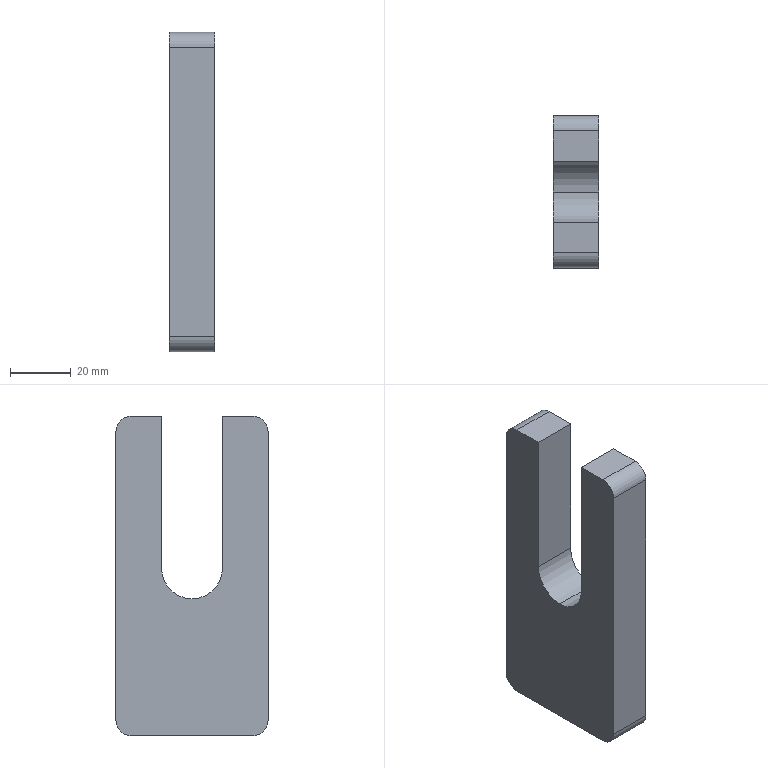Part | SolidWorks | features BaseBody 1 | 1 solid | 15 faces | box 15 x 50 x 105 mm | volume 61072 mm3 | plane 9 | cylinder 6 | commonest cylinder face diameters 10 x4 20 x2
STEP:
#1=CARTESIAN_POINT('',(0.,25.,-60.));
#2=VERTEX_POINT('',#1);
#3=CARTESIAN_POINT('',(0.,35.,-50.));
#4=VERTEX_POINT('',#3);
#5=CARTESIAN_POINT('',(0.,25.,-50.));
#6=DIRECTION('',(1.,0.,0.));
#7=DIRECTION('',(0.,0.,-1.));
#8=AXIS2_PLACEMENT_3D('',#5,#6,#7);
#9=CIRCLE('',#8,10.);
#10=EDGE_CURVE('',#2,#4,#9,.T.);
#11=ORIENTED_EDGE('',*,*,#10,.F.);
#12=CARTESIAN_POINT('',(15.,25.,-60.));
#13=VERTEX_POINT('',#12);
#14=CARTESIAN_POINT('',(0.,25.,-60.));
#15=DIRECTION('',(1.,0.,0.));
#16=VECTOR('',#15,1000.);
#17=LINE('',#14,#16);
#18=EDGE_CURVE('',#2,#13,#17,.T.);
#19=ORIENTED_EDGE('',*,*,#18,.T.);
#20=CARTESIAN_POINT('',(15.,35.,-50.));
#21=VERTEX_POINT('',#20);
#22=CARTESIAN_POINT('',(15.,25.,-50.));
#23=DIRECTION('',(-1.,0.,0.));
#24=DIRECTION('',(0.,0.,-1.));
#25=AXIS2_PLACEMENT_3D('',#22,#23,#24);
#26=CIRCLE('',#25,10.);
#27=EDGE_CURVE('',#21,#13,#26,.T.);
#28=ORIENTED_EDGE('',*,*,#27,.F.);
#29=CARTESIAN_POINT('',(0.,35.,-50.));
#30=DIRECTION('',(1.,0.,0.));
#31=VECTOR('',#30,1000.);
#32=LINE('',#29,#31);
#33=EDGE_CURVE('',#4,#21,#32,.T.);
#34=ORIENTED_EDGE('',*,*,#33,.F.);
#35=EDGE_LOOP('',(#11,#19,#28,#34));
#36=FACE_OUTER_BOUND('',#35,.T.);
#37=CARTESIAN_POINT('',(0.,25.,-50.));
#38=DIRECTION('',(1.,0.,0.));
#39=DIRECTION('',(0.,0.,-1.));
#40=AXIS2_PLACEMENT_3D('',#37,#38,#39);
#41=CYLINDRICAL_SURFACE('',#40,10.);
#42=ADVANCED_FACE('',(#36),#41,.F.);
#43=CARTESIAN_POINT('',(0.,15.,-50.));
#44=VERTEX_POINT('',#43);
#45=CARTESIAN_POINT('',(0.,25.,-50.));
#46=DIRECTION('',(1.,0.,0.));
#47=DIRECTION('',(0.,0.,-1.));
#48=AXIS2_PLACEMENT_3D('',#45,#46,#47);
#49=CIRCLE('',#48,10.);
#50=EDGE_CURVE('',#44,#2,#49,.T.);
#51=ORIENTED_EDGE('',*,*,#50,.T.);
#52=ORIENTED_EDGE('',*,*,#10,.T.);
#53=CARTESIAN_POINT('',(0.,35.,0.));
#54=VERTEX_POINT('',#53);
#55=CARTESIAN_POINT('',(0.,35.,0.));
#56=DIRECTION('',(0.,0.,1.));
#57=VECTOR('',#56,1000.);
#58=LINE('',#55,#57);
#59=EDGE_CURVE('',#4,#54,#58,.T.);
#60=ORIENTED_EDGE('',*,*,#59,.T.);
#61=CARTESIAN_POINT('',(0.,45.,0.));
#62=VERTEX_POINT('',#61);
#63=CARTESIAN_POINT('',(0.,0.,0.));
#64=DIRECTION('',(0.,1.,0.));
#65=VECTOR('',#64,1000.);
#66=LINE('',#63,#65);
#67=EDGE_CURVE('',#54,#62,#66,.T.);
#68=ORIENTED_EDGE('',*,*,#67,.T.);
#69=CARTESIAN_POINT('',(0.,50.,-5.));
#70=VERTEX_POINT('',#69);
#71=CARTESIAN_POINT('',(0.,45.,-5.));
#72=DIRECTION('',(-1.,0.,0.));
#73=DIRECTION('',(0.,0.,1.));
#74=AXIS2_PLACEMENT_3D('',#71,#72,#73);
#75=CIRCLE('',#74,5.);
#76=EDGE_CURVE('',#62,#70,#75,.T.);
#77=ORIENTED_EDGE('',*,*,#76,.T.);
#78=CARTESIAN_POINT('',(0.,50.,-100.));
#79=VERTEX_POINT('',#78);
#80=CARTESIAN_POINT('',(0.,50.,0.));
#81=DIRECTION('',(0.,0.,-1.));
#82=VECTOR('',#81,1000.);
#83=LINE('',#80,#82);
#84=EDGE_CURVE('',#70,#79,#83,.T.);
#85=ORIENTED_EDGE('',*,*,#84,.T.);
#86=CARTESIAN_POINT('',(0.,45.,-105.));
#87=VERTEX_POINT('',#86);
#88=CARTESIAN_POINT('',(0.,45.,-100.));
#89=DIRECTION('',(-1.,0.,0.));
#90=DIRECTION('',(0.,0.,1.));
#91=AXIS2_PLACEMENT_3D('',#88,#89,#90);
#92=CIRCLE('',#91,5.);
#93=EDGE_CURVE('',#79,#87,#92,.T.);
#94=ORIENTED_EDGE('',*,*,#93,.T.);
#95=CARTESIAN_POINT('',(0.,5.,-105.));
#96=VERTEX_POINT('',#95);
#97=CARTESIAN_POINT('',(0.,0.,-105.));
#98=DIRECTION('',(0.,-1.,0.));
#99=VECTOR('',#98,1000.);
#100=LINE('',#97,#99);
#101=EDGE_CURVE('',#87,#96,#100,.T.);
#102=ORIENTED_EDGE('',*,*,#101,.T.);
#103=CARTESIAN_POINT('',(0.,0.,-100.));
#104=VERTEX_POINT('',#103);
#105=CARTESIAN_POINT('',(0.,5.,-100.));
#106=DIRECTION('',(-1.,0.,0.));
#107=DIRECTION('',(0.,0.,1.));
#108=AXIS2_PLACEMENT_3D('',#105,#106,#107);
#109=CIRCLE('',#108,5.);
#110=EDGE_CURVE('',#96,#104,#109,.T.);
#111=ORIENTED_EDGE('',*,*,#110,.T.);
#112=CARTESIAN_POINT('',(0.,0.,-5.));
#113=VERTEX_POINT('',#112);
#114=CARTESIAN_POINT('',(0.,0.,0.));
#115=DIRECTION('',(0.,0.,1.));
#116=VECTOR('',#115,1000.);
#117=LINE('',#114,#116);
#118=EDGE_CURVE('',#104,#113,#117,.T.);
#119=ORIENTED_EDGE('',*,*,#118,.T.);
#120=CARTESIAN_POINT('',(0.,5.,0.));
#121=VERTEX_POINT('',#120);
#122=CARTESIAN_POINT('',(0.,5.,-5.));
#123=DIRECTION('',(-1.,0.,0.));
#124=DIRECTION('',(0.,0.,1.));
#125=AXIS2_PLACEMENT_3D('',#122,#123,#124);
#126=CIRCLE('',#125,5.);
#127=EDGE_CURVE('',#113,#121,#126,.T.);
#128=ORIENTED_EDGE('',*,*,#127,.T.);
#129=CARTESIAN_POINT('',(0.,15.,0.));
#130=VERTEX_POINT('',#129);
#131=CARTESIAN_POINT('',(0.,0.,0.));
#132=DIRECTION('',(0.,1.,0.));
#133=VECTOR('',#132,1000.);
#134=LINE('',#131,#133);
#135=EDGE_CURVE('',#121,#130,#134,.T.);
#136=ORIENTED_EDGE('',*,*,#135,.T.);
#137=CARTESIAN_POINT('',(0.,15.,0.));
#138=DIRECTION('',(0.,0.,-1.));
#139=VECTOR('',#138,1000.);
#140=LINE('',#137,#139);
#141=EDGE_CURVE('',#130,#44,#140,.T.);
#142=ORIENTED_EDGE('',*,*,#141,.T.);
#143=EDGE_LOOP('',(#51,#52,#60,#68,#77,#85,#94,#102,#111,#119,#128,#136,#142));
#144=FACE_OUTER_BOUND('',#143,.T.);
#145=CARTESIAN_POINT('',(0.,0.,0.));
#146=DIRECTION('',(-1.,0.,0.));
#147=DIRECTION('',(0.,0.,1.));
#148=AXIS2_PLACEMENT_3D('',#145,#146,#147);
#149=PLANE('',#148);
#150=ADVANCED_FACE('',(#144),#149,.T.);
#151=ORIENTED_EDGE('',*,*,#18,.F.);
#152=ORIENTED_EDGE('',*,*,#50,.F.);
#153=CARTESIAN_POINT('',(15.,15.,-50.));
#154=VERTEX_POINT('',#153);
#155=CARTESIAN_POINT('',(0.,15.,-50.));
#156=DIRECTION('',(-1.,0.,0.));
#157=VECTOR('',#156,1000.);
#158=LINE('',#155,#157);
#159=EDGE_CURVE('',#154,#44,#158,.T.);
#160=ORIENTED_EDGE('',*,*,#159,.F.);
#161=CARTESIAN_POINT('',(15.,25.,-50.));
#162=DIRECTION('',(-1.,0.,0.));
#163=DIRECTION('',(0.,0.,-1.));
#164=AXIS2_PLACEMENT_3D('',#161,#162,#163);
#165=CIRCLE('',#164,10.);
#166=EDGE_CURVE('',#13,#154,#165,.T.);
#167=ORIENTED_EDGE('',*,*,#166,.F.);
#168=EDGE_LOOP('',(#151,#152,#160,#167));
#169=FACE_OUTER_BOUND('',#168,.T.);
#170=CARTESIAN_POINT('',(0.,25.,-50.));
#171=DIRECTION('',(1.,0.,0.));
#172=DIRECTION('',(0.,0.,-1.));
#173=AXIS2_PLACEMENT_3D('',#170,#171,#172);
#174=CYLINDRICAL_SURFACE('',#173,10.);
#175=ADVANCED_FACE('',(#169),#174,.F.);
#176=ORIENTED_EDGE('',*,*,#159,.T.);
#177=ORIENTED_EDGE('',*,*,#141,.F.);
#178=CARTESIAN_POINT('',(15.,15.,0.));
#179=VERTEX_POINT('',#178);
#180=CARTESIAN_POINT('',(0.,15.,0.));
#181=DIRECTION('',(-1.,0.,0.));
#182=VECTOR('',#181,1000.);
#183=LINE('',#180,#182);
#184=EDGE_CURVE('',#179,#130,#183,.T.);
#185=ORIENTED_EDGE('',*,*,#184,.F.);
#186=CARTESIAN_POINT('',(15.,15.,0.));
#187=DIRECTION('',(0.,0.,1.));
#188=VECTOR('',#187,1000.);
#189=LINE('',#186,#188);
#190=EDGE_CURVE('',#154,#179,#189,.T.);
#191=ORIENTED_EDGE('',*,*,#190,.F.);
#192=EDGE_LOOP('',(#176,#177,#185,#191));
#193=FACE_OUTER_BOUND('',#192,.T.);
#194=CARTESIAN_POINT('',(0.,15.,0.));
#195=DIRECTION('',(0.,-1.,0.));
#196=DIRECTION('',(0.,0.,-1.));
#197=AXIS2_PLACEMENT_3D('',#194,#195,#196);
#198=PLANE('',#197);
#199=ADVANCED_FACE('',(#193),#198,.F.);
#200=ORIENTED_EDGE('',*,*,#184,.T.);
#201=ORIENTED_EDGE('',*,*,#135,.F.);
#202=CARTESIAN_POINT('',(15.,5.,0.));
#203=VERTEX_POINT('',#202);
#204=CARTESIAN_POINT('',(15.,5.,0.));
#205=DIRECTION('',(-1.,0.,0.));
#206=VECTOR('',#205,1000.);
#207=LINE('',#204,#206);
#208=EDGE_CURVE('',#203,#121,#207,.T.);
#209=ORIENTED_EDGE('',*,*,#208,.F.);
#210=CARTESIAN_POINT('',(15.,0.,0.));
#211=DIRECTION('',(0.,-1.,0.));
#212=VECTOR('',#211,1000.);
#213=LINE('',#210,#212);
#214=EDGE_CURVE('',#179,#203,#213,.T.);
#215=ORIENTED_EDGE('',*,*,#214,.F.);
#216=EDGE_LOOP('',(#200,#201,#209,#215));
#217=FACE_OUTER_BOUND('',#216,.T.);
#218=CARTESIAN_POINT('',(15.,0.,0.));
#219=DIRECTION('',(0.,0.,-1.));
#220=DIRECTION('',(-1.,0.,0.));
#221=AXIS2_PLACEMENT_3D('',#218,#219,#220);
#222=PLANE('',#221);
#223=ADVANCED_FACE('',(#217),#222,.F.);
#224=ORIENTED_EDGE('',*,*,#127,.F.);
#225=CARTESIAN_POINT('',(15.,0.,-5.));
#226=VERTEX_POINT('',#225);
#227=CARTESIAN_POINT('',(15.,0.,-5.));
#228=DIRECTION('',(1.,0.,0.));
#229=VECTOR('',#228,1000.);
#230=LINE('',#227,#229);
#231=EDGE_CURVE('',#113,#226,#230,.T.);
#232=ORIENTED_EDGE('',*,*,#231,.T.);
#233=CARTESIAN_POINT('',(15.,5.,-5.));
#234=DIRECTION('',(-1.,0.,0.));
#235=DIRECTION('',(0.,0.,1.));
#236=AXIS2_PLACEMENT_3D('',#233,#234,#235);
#237=CIRCLE('',#236,5.);
#238=EDGE_CURVE('',#226,#203,#237,.T.);
#239=ORIENTED_EDGE('',*,*,#238,.T.);
#240=ORIENTED_EDGE('',*,*,#208,.T.);
#241=EDGE_LOOP('',(#224,#232,#239,#240));
#242=FACE_OUTER_BOUND('',#241,.T.);
#243=CARTESIAN_POINT('',(15.,5.,-5.));
#244=DIRECTION('',(-1.,0.,0.));
#245=DIRECTION('',(0.,0.,1.));
#246=AXIS2_PLACEMENT_3D('',#243,#244,#245);
#247=CYLINDRICAL_SURFACE('',#246,5.);
#248=ADVANCED_FACE('',(#242),#247,.T.);
#249=CARTESIAN_POINT('',(15.,0.,-100.));
#250=VERTEX_POINT('',#249);
#251=CARTESIAN_POINT('',(15.,0.,-100.));
#252=DIRECTION('',(-1.,0.,0.));
#253=VECTOR('',#252,1000.);
#254=LINE('',#251,#253);
#255=EDGE_CURVE('',#250,#104,#254,.T.);
#256=ORIENTED_EDGE('',*,*,#255,.F.);
#257=CARTESIAN_POINT('',(15.,0.,0.));
#258=DIRECTION('',(0.,0.,-1.));
#259=VECTOR('',#258,1000.);
#260=LINE('',#257,#259);
#261=EDGE_CURVE('',#226,#250,#260,.T.);
#262=ORIENTED_EDGE('',*,*,#261,.F.);
#263=ORIENTED_EDGE('',*,*,#231,.F.);
#264=ORIENTED_EDGE('',*,*,#118,.F.);
#265=EDGE_LOOP('',(#256,#262,#263,#264));
#266=FACE_OUTER_BOUND('',#265,.T.);
#267=CARTESIAN_POINT('',(15.,0.,0.));
#268=DIRECTION('',(0.,1.,0.));
#269=DIRECTION('',(0.,0.,1.));
#270=AXIS2_PLACEMENT_3D('',#267,#268,#269);
#271=PLANE('',#270);
#272=ADVANCED_FACE('',(#266),#271,.F.);
#273=ORIENTED_EDGE('',*,*,#110,.F.);
#274=CARTESIAN_POINT('',(15.,5.,-105.));
#275=VERTEX_POINT('',#274);
#276=CARTESIAN_POINT('',(15.,5.,-105.));
#277=DIRECTION('',(1.,0.,0.));
#278=VECTOR('',#277,1000.);
#279=LINE('',#276,#278);
#280=EDGE_CURVE('',#96,#275,#279,.T.);
#281=ORIENTED_EDGE('',*,*,#280,.T.);
#282=CARTESIAN_POINT('',(15.,5.,-100.));
#283=DIRECTION('',(-1.,0.,0.));
#284=DIRECTION('',(0.,0.,1.));
#285=AXIS2_PLACEMENT_3D('',#282,#283,#284);
#286=CIRCLE('',#285,5.);
#287=EDGE_CURVE('',#275,#250,#286,.T.);
#288=ORIENTED_EDGE('',*,*,#287,.T.);
#289=ORIENTED_EDGE('',*,*,#255,.T.);
#290=EDGE_LOOP('',(#273,#281,#288,#289));
#291=FACE_OUTER_BOUND('',#290,.T.);
#292=CARTESIAN_POINT('',(15.,5.,-100.));
#293=DIRECTION('',(-1.,0.,0.));
#294=DIRECTION('',(0.,0.,1.));
#295=AXIS2_PLACEMENT_3D('',#292,#293,#294);
#296=CYLINDRICAL_SURFACE('',#295,5.);
#297=ADVANCED_FACE('',(#291),#296,.T.);
#298=ORIENTED_EDGE('',*,*,#280,.F.);
#299=ORIENTED_EDGE('',*,*,#101,.F.);
#300=CARTESIAN_POINT('',(15.,45.,-105.));
#301=VERTEX_POINT('',#300);
#302=CARTESIAN_POINT('',(15.,45.,-105.));
#303=DIRECTION('',(-1.,0.,0.));
#304=VECTOR('',#303,1000.);
#305=LINE('',#302,#304);
#306=EDGE_CURVE('',#301,#87,#305,.T.);
#307=ORIENTED_EDGE('',*,*,#306,.F.);
#308=CARTESIAN_POINT('',(15.,0.,-105.));
#309=DIRECTION('',(0.,1.,0.));
#310=VECTOR('',#309,1000.);
#311=LINE('',#308,#310);
#312=EDGE_CURVE('',#275,#301,#311,.T.);
#313=ORIENTED_EDGE('',*,*,#312,.F.);
#314=EDGE_LOOP('',(#298,#299,#307,#313));
#315=FACE_OUTER_BOUND('',#314,.T.);
#316=CARTESIAN_POINT('',(15.,0.,-105.));
#317=DIRECTION('',(0.,0.,1.));
#318=DIRECTION('',(1.,0.,0.));
#319=AXIS2_PLACEMENT_3D('',#316,#317,#318);
#320=PLANE('',#319);
#321=ADVANCED_FACE('',(#315),#320,.F.);
#322=ORIENTED_EDGE('',*,*,#93,.F.);
#323=CARTESIAN_POINT('',(15.,50.,-100.));
#324=VERTEX_POINT('',#323);
#325=CARTESIAN_POINT('',(15.,50.,-100.));
#326=DIRECTION('',(1.,0.,0.));
#327=VECTOR('',#326,1000.);
#328=LINE('',#325,#327);
#329=EDGE_CURVE('',#79,#324,#328,.T.);
#330=ORIENTED_EDGE('',*,*,#329,.T.);
#331=CARTESIAN_POINT('',(15.,45.,-100.));
#332=DIRECTION('',(-1.,0.,0.));
#333=DIRECTION('',(0.,0.,1.));
#334=AXIS2_PLACEMENT_3D('',#331,#332,#333);
#335=CIRCLE('',#334,5.);
#336=EDGE_CURVE('',#324,#301,#335,.T.);
#337=ORIENTED_EDGE('',*,*,#336,.T.);
#338=ORIENTED_EDGE('',*,*,#306,.T.);
#339=EDGE_LOOP('',(#322,#330,#337,#338));
#340=FACE_OUTER_BOUND('',#339,.T.);
#341=CARTESIAN_POINT('',(15.,45.,-100.));
#342=DIRECTION('',(-1.,0.,0.));
#343=DIRECTION('',(0.,0.,1.));
#344=AXIS2_PLACEMENT_3D('',#341,#342,#343);
#345=CYLINDRICAL_SURFACE('',#344,5.);
#346=ADVANCED_FACE('',(#340),#345,.T.);
#347=ORIENTED_EDGE('',*,*,#329,.F.);
#348=ORIENTED_EDGE('',*,*,#84,.F.);
#349=CARTESIAN_POINT('',(15.,50.,-5.));
#350=VERTEX_POINT('',#349);
#351=CARTESIAN_POINT('',(15.,50.,-5.));
#352=DIRECTION('',(-1.,0.,0.));
#353=VECTOR('',#352,1000.);
#354=LINE('',#351,#353);
#355=EDGE_CURVE('',#350,#70,#354,.T.);
#356=ORIENTED_EDGE('',*,*,#355,.F.);
#357=CARTESIAN_POINT('',(15.,50.,0.));
#358=DIRECTION('',(0.,0.,1.));
#359=VECTOR('',#358,1000.);
#360=LINE('',#357,#359);
#361=EDGE_CURVE('',#324,#350,#360,.T.);
#362=ORIENTED_EDGE('',*,*,#361,.F.);
#363=EDGE_LOOP('',(#347,#348,#356,#362));
#364=FACE_OUTER_BOUND('',#363,.T.);
#365=CARTESIAN_POINT('',(15.,50.,0.));
#366=DIRECTION('',(0.,-1.,0.));
#367=DIRECTION('',(0.,0.,-1.));
#368=AXIS2_PLACEMENT_3D('',#365,#366,#367);
#369=PLANE('',#368);
#370=ADVANCED_FACE('',(#364),#369,.F.);
#371=ORIENTED_EDGE('',*,*,#76,.F.);
#372=CARTESIAN_POINT('',(15.,45.,0.));
#373=VERTEX_POINT('',#372);
#374=CARTESIAN_POINT('',(15.,45.,0.));
#375=DIRECTION('',(1.,0.,0.));
#376=VECTOR('',#375,1000.);
#377=LINE('',#374,#376);
#378=EDGE_CURVE('',#62,#373,#377,.T.);
#379=ORIENTED_EDGE('',*,*,#378,.T.);
#380=CARTESIAN_POINT('',(15.,45.,-5.));
#381=DIRECTION('',(-1.,0.,0.));
#382=DIRECTION('',(0.,0.,1.));
#383=AXIS2_PLACEMENT_3D('',#380,#381,#382);
#384=CIRCLE('',#383,5.);
#385=EDGE_CURVE('',#373,#350,#384,.T.);
#386=ORIENTED_EDGE('',*,*,#385,.T.);
#387=ORIENTED_EDGE('',*,*,#355,.T.);
#388=EDGE_LOOP('',(#371,#379,#386,#387));
#389=FACE_OUTER_BOUND('',#388,.T.);
#390=CARTESIAN_POINT('',(15.,45.,-5.));
#391=DIRECTION('',(-1.,0.,0.));
#392=DIRECTION('',(0.,0.,1.));
#393=AXIS2_PLACEMENT_3D('',#390,#391,#392);
#394=CYLINDRICAL_SURFACE('',#393,5.);
#395=ADVANCED_FACE('',(#389),#394,.T.);
#396=CARTESIAN_POINT('',(15.,35.,0.));
#397=VERTEX_POINT('',#396);
#398=CARTESIAN_POINT('',(15.,35.,0.));
#399=DIRECTION('',(-1.,0.,0.));
#400=VECTOR('',#399,1000.);
#401=LINE('',#398,#400);
#402=EDGE_CURVE('',#397,#54,#401,.T.);
#403=ORIENTED_EDGE('',*,*,#402,.F.);
#404=CARTESIAN_POINT('',(15.,0.,0.));
#405=DIRECTION('',(0.,-1.,0.));
#406=VECTOR('',#405,1000.);
#407=LINE('',#404,#406);
#408=EDGE_CURVE('',#373,#397,#407,.T.);
#409=ORIENTED_EDGE('',*,*,#408,.F.);
#410=ORIENTED_EDGE('',*,*,#378,.F.);
#411=ORIENTED_EDGE('',*,*,#67,.F.);
#412=EDGE_LOOP('',(#403,#409,#410,#411));
#413=FACE_OUTER_BOUND('',#412,.T.);
#414=CARTESIAN_POINT('',(15.,0.,0.));
#415=DIRECTION('',(0.,0.,-1.));
#416=DIRECTION('',(-1.,0.,0.));
#417=AXIS2_PLACEMENT_3D('',#414,#415,#416);
#418=PLANE('',#417);
#419=ADVANCED_FACE('',(#413),#418,.F.);
#420=ORIENTED_EDGE('',*,*,#402,.T.);
#421=ORIENTED_EDGE('',*,*,#59,.F.);
#422=ORIENTED_EDGE('',*,*,#33,.T.);
#423=CARTESIAN_POINT('',(15.,35.,0.));
#424=DIRECTION('',(0.,0.,-1.));
#425=VECTOR('',#424,1000.);
#426=LINE('',#423,#425);
#427=EDGE_CURVE('',#397,#21,#426,.T.);
#428=ORIENTED_EDGE('',*,*,#427,.F.);
#429=EDGE_LOOP('',(#420,#421,#422,#428));
#430=FACE_OUTER_BOUND('',#429,.T.);
#431=CARTESIAN_POINT('',(0.,35.,0.));
#432=DIRECTION('',(0.,1.,0.));
#433=DIRECTION('',(0.,0.,1.));
#434=AXIS2_PLACEMENT_3D('',#431,#432,#433);
#435=PLANE('',#434);
#436=ADVANCED_FACE('',(#430),#435,.F.);
#437=ORIENTED_EDGE('',*,*,#427,.T.);
#438=ORIENTED_EDGE('',*,*,#27,.T.);
#439=ORIENTED_EDGE('',*,*,#166,.T.);
#440=ORIENTED_EDGE('',*,*,#190,.T.);
#441=ORIENTED_EDGE('',*,*,#214,.T.);
#442=ORIENTED_EDGE('',*,*,#238,.F.);
#443=ORIENTED_EDGE('',*,*,#261,.T.);
#444=ORIENTED_EDGE('',*,*,#287,.F.);
#445=ORIENTED_EDGE('',*,*,#312,.T.);
#446=ORIENTED_EDGE('',*,*,#336,.F.);
#447=ORIENTED_EDGE('',*,*,#361,.T.);
#448=ORIENTED_EDGE('',*,*,#385,.F.);
#449=ORIENTED_EDGE('',*,*,#408,.T.);
#450=EDGE_LOOP('',(#437,#438,#439,#440,#441,#442,#443,#444,#445,#446,#447,#448,#449));
#451=FACE_OUTER_BOUND('',#450,.T.);
#452=CARTESIAN_POINT('',(15.,0.,0.));
#453=DIRECTION('',(-1.,0.,0.));
#454=DIRECTION('',(0.,0.,1.));
#455=AXIS2_PLACEMENT_3D('',#452,#453,#454);
#456=PLANE('',#455);
#457=ADVANCED_FACE('',(#451),#456,.F.);
#458=CLOSED_SHELL('',(#42,#150,#175,#199,#223,#248,#272,#297,#321,#346,#370,#395,#419,#436,#457));
#459=MANIFOLD_SOLID_BREP('',#458);
#460=CARTESIAN_POINT('',(0.,0.,0.));
#461=DIRECTION('',(0.,0.,1.));
#462=DIRECTION('',(1.,0.,0.));
#463=AXIS2_PLACEMENT_3D('',#460,#461,#462);
#464=(LENGTH_UNIT()NAMED_UNIT(*)SI_UNIT(.MILLI.,.METRE.));
#465=UNCERTAINTY_MEASURE_WITH_UNIT(LENGTH_MEASURE(0.00001),#464,'','');
#466=(NAMED_UNIT(*)PLANE_ANGLE_UNIT()SI_UNIT($,.RADIAN.));
#467=(NAMED_UNIT(*)SI_UNIT($,.STERADIAN.)SOLID_ANGLE_UNIT());
#468=(GEOMETRIC_REPRESENTATION_CONTEXT(3)GLOBAL_UNCERTAINTY_ASSIGNED_CONTEXT((#465))GLOBAL_UNIT_ASSIGNED_CONTEXT((#464,#466,#467))REPRESENTATION_CONTEXT('',''));
#469=ADVANCED_BREP_SHAPE_REPRESENTATION('',(#459,#463),#468);